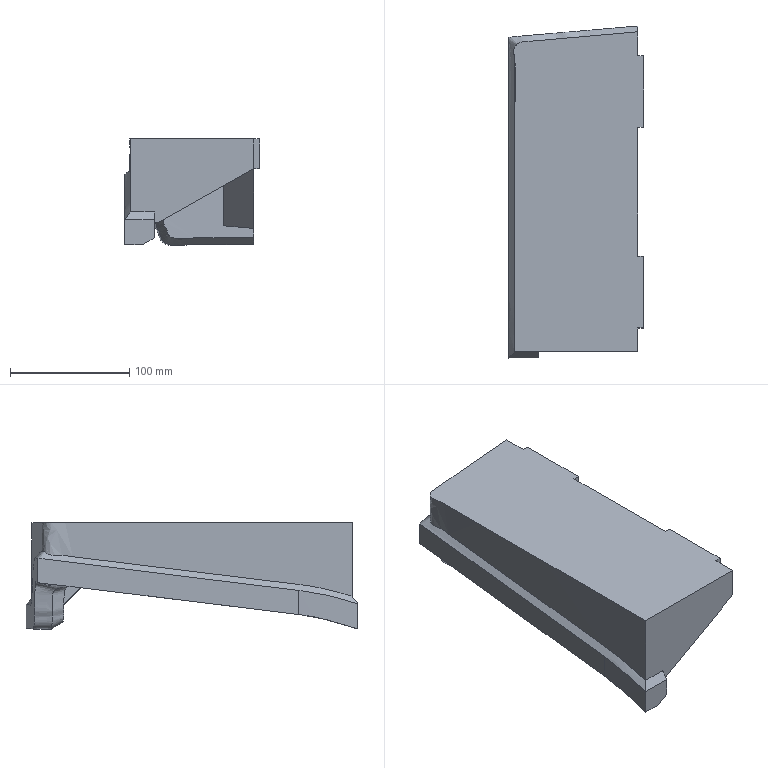Part | NX | features solid 2 | 1 solid | 37 faces | box 113.083 x 278.029 x 89.003 mm | volume 1116165 mm3 | plane 25 | spline 7 | cylinder 5 | commonest cylinder face diameters 30 x5